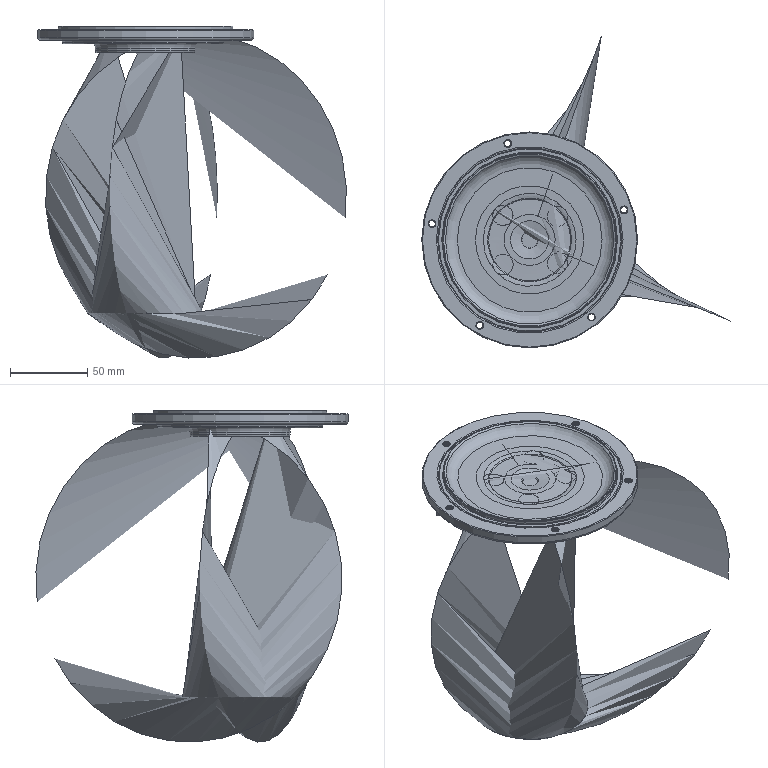NC program | NX | posted with a generic post
Lines 31 to 990 of 33119:
(FIXED_CONTOUR , TOOL : D6R0.5)
N60 T05 M6
N62 G17 G43 G0 G90 X-53.25 Y-3. Z30. S9500 H5 M3
N64 Z3.6
N66 G94 G1 Z2.996 F1000.
N68 Y-2.963 Z2.527
N70 X-53.249 Y-2.853 Z2.069
N72 X-53.246 Y-2.673 Z1.634
N74 X-53.243 Y-2.427 Z1.233
N76 X-53.24 Y-2.121 Z0.875
N78 X-53.235 Y-1.763 Z0.569
N80 X-53.23 Y-1.362 Z0.323
N82 X-53.225 Y-0.927 Z0.143
N84 X-53.219 Y-0.469 Z0.033
N86 X-53.214 Y0. Z-0.004
N88 G2 X29.564 Y44.245 R53.214 F3500.
N90 G1 X30.641 Y43.507
N92 G2 X19.151 Y-49.648 R53.214
N94 G1 X17.927 Y-50.103
N96 G2 X-53.198 Y-1.306 R53.214
N98 G1 X-53.214 Y0.
N100 G2 X-46.923 Y25.081 R53.21
N102 G1 X-46.293 Y26.225
N104 G2 X-28.461 Y44.944 R53.202
N106 G1 X-27.349 Y45.629 Z-0.005
N108 G2 X-2.61 Y53.126 R53.193
N110 G1 X-1.305 Y53.173 Z-0.006
N112 G2 X25.069 Y46.902 R53.185
N114 G1 X26.213 Y46.272
N116 G2 X44.923 Y28.447 R53.177
N118 G1 X45.608 Y27.336 Z-0.007
N120 G2 X53.101 Y2.609 R53.169
N122 G1 X53.149 Y1.305
N124 G2 X47.481 Y-23.9 R53.161
N126 G1 X46.88 Y-25.058 Z-0.008
N128 G2 X28.434 Y-44.903 R53.152
N130 G1 X27.324 Y-45.587
N132 G2 X2.607 Y-53.076 R53.144
N134 G1 X1.304 Y-53.124 Z-0.009
N136 G2 X-23.889 Y-47.459 R53.136
N138 G1 X-25.046 Y-46.858
N140 G2 X-44.171 Y-29.514 R53.128
N142 G1 X-44.882 Y-28.421 Z-0.01
N144 G2 X-52.972 Y-3.907 R53.12
N146 G1 X-53.052 Y-2.606
N148 G2 X-48.009 Y22.707 R53.112
N150 G1 X-47.437 Y23.878 Z-0.011
N152 G2 X-30.575 Y43.414 R53.104
N154 G1 X-29.5 Y44.151
N156 G2 X-5.204 Y52.836 R53.096
N158 G1 X-3.906 Y52.947 Z-0.012
N160 G2 X21.512 Y48.53 R53.087
N162 G1 X22.696 Y47.987
N164 G2 X42.631 Y31.617 R53.079
N166 G1 X43.393 Y30.561 Z-0.013
N168 G2 X52.493 Y7.787 R53.071
N170 G1 X52.668 Y6.496
N172 G2 X51.139 Y-14.152 R53.064
N174 G1 X50.776 Y-15.403 Z-0.014
N176 G2 X42.614 Y-31.605 R53.058
N178 G1 X41.826 Y-32.641
N180 G2 X30.547 Y-43.373 R53.053
N182 G1 X29.473 Y-44.109 Z-0.015
N184 G2 X16.64 Y-50.368 R53.048
N186 G1 X15.398 Y-50.761
N188 G2 X2.603 Y-52.978 R53.043
N190 G1 X1.302 Y-53.025 Z-0.016
N192 G2 X-10.347 Y-52.019 R53.039
N194 G1 X-11.621 Y-51.749
N196 G2 X-22.675 Y-47.942 R53.036
N198 G1 X-23.844 Y-47.371 Z-0.017
N200 G2 X-32.626 Y-41.806 R53.032
N202 G1 X-33.642 Y-40.993
N204 G2 X-40.99 Y-33.64 R53.028
N206 G1 X-41.803 Y-32.624 Z-0.018
N208 G2 X-47.362 Y-23.84 R53.025
N210 G1 X-47.932 Y-22.67
N212 G2 X-51.1 Y-14.141 R53.022
N214 G1 X-51.431 Y-12.883 Z-0.019
N216 G2 X-52.874 Y-3.9 R53.019
N218 G1 X-52.953 Y-2.601 Z-0.02
N220 G2 X-52.615 Y6.489 R53.016
N222 G1 X-52.44 Y7.779
N224 G2 X-50.729 Y15.388 R53.013
N226 G1 X-50.335 Y16.629 Z-0.021
N228 G2 X-47.349 Y23.833 R53.01
N230 G1 X-46.749 Y24.988
N232 G2 X-42.575 Y31.576 R53.007
N234 G1 X-41.787 Y32.611 Z-0.022
N236 G2 X-36.548 Y38.388 R53.004
N238 G1 X-35.595 Y39.273
N240 G2 X-29.446 Y44.068 R53.002
N242 G1 X-28.355 Y44.777 Z-0.023
N244 G2 X-21.477 Y48.451 R52.999
N246 G1 X-20.281 Y48.963
N248 G2 X-12.877 Y51.407 R52.996
N250 G1 X-11.611 Y51.707 Z-0.024
N252 G2 X-3.898 Y52.849 R52.994
N254 G1 X-2.6 Y52.928
N256 G2 X5.194 Y52.735 R52.991
N258 G1 X6.486 Y52.591 Z-0.025
N260 G2 X14.132 Y51.068 R52.988
N262 G1 X15.381 Y50.705
N264 G2 X22.654 Y47.897 R52.986
N266 G1 X23.822 Y47.327 Z-0.026
N268 G2 X30.507 Y43.317 R52.983
N270 G1 X31.561 Y42.555
N272 G2 X37.462 Y37.462 R52.98
N274 G1 X38.37 Y36.531 Z-0.027
N276 G2 X43.313 Y30.504 R52.977
N278 G1 X44.048 Y29.432
N280 G2 X47.888 Y22.649 R52.975
N282 G1 X48.429 Y21.467 Z-0.028
N284 G2 X51.052 Y14.128 R52.972
N286 G1 X51.383 Y12.871
N288 G2 X52.713 Y5.192 R52.969
N290 G1 X52.824 Y3.897 Z-0.029
N292 G2 X52.822 Y-3.896 R52.967
N294 G1 X52.71 Y-5.191
N296 G2 X51.376 Y-12.869 R52.964
N298 G1 X51.044 Y-14.126 Z-0.03
N300 G2 X48.417 Y-21.462 R52.961
N302 G1 X47.875 Y-22.643
N304 G2 X44.032 Y-29.422 R52.959
N306 G1 X43.297 Y-30.493 Z-0.031
N308 G2 X38.352 Y-36.514 R52.956
N310 G1 X37.444 Y-37.444
N312 G2 X31.543 Y-42.531 R52.953
N314 G1 X30.49 Y-43.292 Z-0.032
N316 G2 X23.807 Y-47.296 R52.95
N318 G1 X22.639 Y-47.865
N320 G2 X15.37 Y-50.667 R52.948
N322 G1 X14.121 Y-51.028 Z-0.033
N324 G2 X6.481 Y-52.546 R52.945
N326 G1 X5.189 Y-52.689
N328 G2 X-2.598 Y-52.877 R52.942
N330 G1 X-3.895 Y-52.797 Z-0.034
N332 G2 X-11.599 Y-51.652 R52.94
N334 G1 X-12.863 Y-51.352
N336 G2 X-20.258 Y-48.906 R52.937
N338 G1 X-21.452 Y-48.394 Z-0.035
N340 G2 X-28.319 Y-44.721 R52.934
N342 G1 X-29.408 Y-44.012 Z-0.036
N344 G2 X-35.546 Y-39.219 R52.932
N346 G1 X-36.497 Y-38.334
N348 G2 X-41.725 Y-32.563 R52.929
N350 G1 X-42.512 Y-31.529 Z-0.037
N352 G2 X-46.676 Y-24.949 R52.926
N354 G1 X-47.274 Y-23.796
N356 G2 X-50.251 Y-16.601 R52.923
N358 G1 X-50.643 Y-15.362 Z-0.038
N360 G2 X-52.347 Y-7.765 R52.921
N362 G1 X-52.521 Y-6.478
N364 G2 X-52.901 Y1.299 R52.918
N366 G1 X-52.853 Y2.596 Z-0.039
N368 G2 X-51.897 Y10.323 R52.915
N370 G1 X-51.628 Y11.593
N372 G2 X-49.366 Y19.043 R52.913
N374 G1 X-48.884 Y20.248 Z-0.04
N376 G2 X-45.381 Y27.201 R52.91
N378 G1 X-44.7 Y28.306
N380 G2 X-40.061 Y34.557 R52.907
N382 G1 X-39.201 Y35.529 Z-0.041
N384 G2 X-33.562 Y40.895 R52.905
N386 G1 X-32.548 Y41.706
N388 G2 X-26.075 Y46.028 R52.902
N390 G1 X-24.937 Y46.654 Z-0.042
N392 G2 X-17.821 Y49.806 R52.899
N394 G1 X-16.593 Y50.228
N396 G2 X-9.043 Y52.117 R52.896
N398 G1 X-7.761 Y52.322 Z-0.043
N400 G2 X0. Y52.893 R52.894
N402 G1 X1.298 Y52.876
N404 G2 X9.042 Y52.111 R52.891
N406 G1 X10.318 Y51.873 Z-0.044
N408 G2 X17.817 Y49.796 R52.888
N410 G1 X19.034 Y49.343
N412 G2 X26.067 Y46.014 R52.886
N414 G1 X27.188 Y45.36 Z-0.045
N416 G2 X33.548 Y40.878 R52.883
N418 G1 X34.541 Y40.042
N420 G2 X40.041 Y34.539 R52.88
N422 G1 X40.876 Y33.546 Z-0.046
N424 G2 X45.354 Y27.184 R52.878
N426 G1 X46.007 Y26.062
N428 G2 X49.331 Y19.029 R52.875
N430 G1 X49.783 Y17.812 Z-0.047
N432 G2 X51.855 Y10.315 R52.872
N434 G1 X52.092 Y9.039
N436 G2 X52.852 Y1.297 R52.869
N438 G1 X52.868 Y0. Z-0.048
N440 G2 X52.293 Y-7.757 R52.867
N442 G1 X52.087 Y-9.038
N444 G2 X50.195 Y-16.582 R52.864
N446 G1 X49.772 Y-17.809 Z-0.049
N448 G2 X46.619 Y-24.918 R52.861
N450 G1 X45.993 Y-26.055
N452 G2 X41.67 Y-32.52 R52.859
N454 G1 X40.859 Y-33.532 Z-0.05
N456 G2 X35.495 Y-39.163 R52.856
N458 G1 X34.523 Y-40.022
N460 G2 X28.276 Y-44.652 R52.853
N462 G1 X27.171 Y-45.332 Z-0.051
N464 G2 X20.225 Y-48.826 R52.851
N466 G1 X19.02 Y-49.308 Z-0.052
N468 G2 X11.579 Y-51.563 R52.848
N470 G1 X10.31 Y-51.831
N472 G2 X2.593 Y-52.78 R52.845
N474 G1 X1.297 Y-52.828 Z-0.053
N476 G2 X-6.468 Y-52.444 R52.842
N478 G1 X-7.753 Y-52.269
N480 G2 X-15.338 Y-50.563 R52.84
N482 G1 X-16.574 Y-50.171 Z-0.054
N484 G2 X-23.756 Y-47.194 R52.837
N486 G1 X-24.906 Y-46.597
N488 G2 X-31.473 Y-42.436 R52.834
N490 G1 X-32.504 Y-41.651 Z-0.055
N492 G2 X-38.262 Y-36.429 R52.832
N494 G1 X-39.145 Y-35.479
N496 G2 X-43.925 Y-29.35 R52.829
N498 G1 X-44.631 Y-28.263 Z-0.056
N500 G2 X-48.293 Y-21.407 R52.826
N502 G1 X-48.804 Y-20.215
N504 G2 X-51.239 Y-12.835 R52.824
N506 G1 X-51.539 Y-11.573 Z-0.057
N508 G2 X-52.677 Y-3.886 R52.821
N510 G1 X-52.756 Y-2.592
N512 G2 X-52.563 Y5.177 R52.818
N514 G1 X-52.419 Y6.465 Z-0.058
N516 G2 X-50.901 Y14.086 R52.815
N518 G1 X-50.54 Y15.331
N520 G2 X-48.281 Y21.402 R52.813
N522 G1 X-47.741 Y22.58 Z-0.059
N524 G2 X-44.616 Y28.253 R52.811
N526 G1 X-43.909 Y29.339
N528 G2 X-39.986 Y34.492 R52.808
N530 G1 X-39.127 Y35.463 Z-0.06
N532 G2 X-34.491 Y39.984 R52.806
N534 G1 X-33.499 Y40.819
N536 G2 X-28.249 Y44.611 R52.804
N538 G1 X-27.146 Y45.29 Z-0.061
N540 G2 X-21.397 Y48.271 R52.801
N542 G1 X-20.206 Y48.781 Z-0.062
N544 G2 X-14.082 Y50.886 R52.799
N546 G1 X-12.829 Y51.215
N548 G2 X-6.463 Y52.399 R52.797
N550 G1 X-5.175 Y52.541 Z-0.063
N552 G2 X1.296 Y52.778 R52.795
N554 G1 X2.59 Y52.729
N556 X3.884 Y52.65
N558 X5.175 Y52.538
N560 X6.462 Y52.395 Z-0.064
N562 X7.746 Y52.22
N564 X9.025 Y52.014
N566 X10.299 Y51.776
N568 X11.566 Y51.508
N570 X12.827 Y51.208
N572 X14.08 Y50.877
N574 X15.324 Y50.516
N576 X16.559 Y50.124
N578 X17.784 Y49.703
N580 X18.998 Y49.251 Z-0.065
N582 X20.201 Y48.769
N584 X21.392 Y48.259
N586 X22.569 Y47.719
N588 X23.733 Y47.15
N590 X24.883 Y46.553
N592 X26.018 Y45.928
N594 X27.137 Y45.276
N596 X28.24 Y44.596
N598 X29.326 Y43.889 Z-0.066
N600 X30.394 Y43.156
N602 X31.443 Y42.396
N604 X32.474 Y41.612
N606 X33.485 Y40.802
N608 X34.476 Y39.968
N610 X35.446 Y39.109
N612 X36.395 Y38.227
N614 X37.322 Y37.322
N616 X38.227 Y36.395 Z-0.067
N618 X39.108 Y35.445
N620 X39.966 Y34.475
N622 X40.799 Y33.483
N624 X41.609 Y32.472
N626 X42.393 Y31.441
N628 X43.151 Y30.39
N630 X43.884 Y29.322
N632 X44.59 Y28.236
N634 X45.269 Y27.133 Z-0.068
N636 X45.921 Y26.014
N638 X46.545 Y24.879
N640 X47.141 Y23.729
N642 X47.709 Y22.565
N644 X48.248 Y21.387
N646 X48.758 Y20.196
N648 X49.239 Y18.993
N650 X49.69 Y17.779
N652 X50.111 Y16.554 Z-0.069
N654 X50.501 Y15.319
N656 X50.862 Y14.075
N658 X51.191 Y12.823
N660 X51.49 Y11.563
N662 X51.758 Y10.295
N664 X51.995 Y9.022
N666 X52.2 Y7.743
N668 X52.374 Y6.46 Z-0.07
N670 X52.517 Y5.172
N672 X52.627 Y3.882
N674 X52.706 Y2.589
N676 X52.754 Y1.295
N678 X52.769 Y0.
N680 X52.753 Y-1.295
N682 X52.705 Y-2.589
N684 X52.625 Y-3.882
N686 X52.514 Y-5.172 Z-0.071
N688 X52.37 Y-6.459
N690 X52.196 Y-7.743
N692 X51.99 Y-9.021
N694 X51.752 Y-10.294
N696 X51.484 Y-11.561
N698 X51.184 Y-12.821
N700 X50.854 Y-14.073
N702 X50.493 Y-15.317 Z-0.072
N704 X50.101 Y-16.551
N706 X49.679 Y-17.776
N708 X49.228 Y-18.989
N710 X48.747 Y-20.192
N712 X48.236 Y-21.382
N714 X47.696 Y-22.559
N716 X47.128 Y-23.722
N718 X46.531 Y-24.872 Z-0.073
N720 X45.907 Y-26.006
N722 X45.254 Y-27.124
N724 X44.575 Y-28.227
N726 X43.868 Y-29.312
N728 X43.135 Y-30.379
N730 X42.377 Y-31.429
N732 X41.592 Y-32.459
N734 X40.783 Y-33.47 Z-0.074
N736 X39.949 Y-34.46
N738 X39.091 Y-35.43
N740 X38.209 Y-36.378
N742 X37.305 Y-37.305
N744 X36.378 Y-38.209
N746 X35.429 Y-39.09
N748 X34.459 Y-39.947
N750 X33.468 Y-40.78 Z-0.075
N752 X32.456 Y-41.589
N754 X31.426 Y-42.373
N756 X30.376 Y-43.131
N758 X29.308 Y-43.863
N760 X28.223 Y-44.569
N762 X27.12 Y-45.248
N764 X26.002 Y-45.899
N766 X24.867 Y-46.523 Z-0.076
N768 X23.718 Y-47.119
N770 X22.554 Y-47.687
N772 X21.377 Y-48.226
N774 X20.187 Y-48.735
N776 X18.985 Y-49.216
N778 X17.771 Y-49.666
N780 X16.547 Y-50.087
N782 X15.312 Y-50.478 Z-0.077
N784 X14.069 Y-50.838
N786 X12.817 Y-51.168
N788 X11.557 Y-51.466
N790 X10.291 Y-51.734
N792 X9.018 Y-51.971
N794 X7.74 Y-52.176
N796 X6.457 Y-52.35
N798 X5.17 Y-52.492 Z-0.078
N800 X3.88 Y-52.603
N802 X2.588 Y-52.682
N804 X1.294 Y-52.729
N806 X0. Y-52.744
N808 X-1.294 Y-52.728
N810 X-2.588 Y-52.68
N812 X-3.88 Y-52.6
N814 X-5.17 Y-52.489 Z-0.079
N816 X-6.456 Y-52.346
N818 X-7.739 Y-52.171
N820 X-9.017 Y-51.965
N822 X-10.289 Y-51.728
N824 X-11.556 Y-51.46
N826 X-12.815 Y-51.16
N828 X-14.067 Y-50.83 Z-0.08
N830 X-15.31 Y-50.469
N832 X-16.543 Y-50.078
N834 X-17.767 Y-49.656
N836 X-18.98 Y-49.205
N838 X-20.182 Y-48.724
N840 X-21.372 Y-48.214
N842 X-22.548 Y-47.674
N844 X-23.711 Y-47.106 Z-0.081
N846 X-24.86 Y-46.51
N848 X-25.994 Y-45.885
N850 X-27.112 Y-45.233
N852 X-28.213 Y-44.554
N854 X-29.298 Y-43.848
N856 X-30.365 Y-43.115
N858 X-31.414 Y-42.357
N860 X-32.444 Y-41.573 Z-0.082
N862 X-33.454 Y-40.764
N864 X-34.444 Y-39.93
N866 X-35.413 Y-39.073
N868 X-36.361 Y-38.191
N870 X-37.287 Y-37.287
N872 X-38.191 Y-36.361
N874 X-39.071 Y-35.412
N876 X-39.928 Y-34.442 Z-0.083
N878 X-40.761 Y-33.452
N880 X-41.57 Y-32.441
N882 X-42.353 Y-31.411
N884 X-43.111 Y-30.362
N886 X-43.843 Y-29.295
N888 X-44.548 Y-28.21
N890 X-45.227 Y-27.108
N892 X-45.878 Y-25.989 Z-0.084
N894 X-46.502 Y-24.856
N896 X-47.097 Y-23.707
N898 X-47.664 Y-22.544
N900 X-48.203 Y-21.367
N902 X-48.712 Y-20.177
N904 X-49.193 Y-18.976
N906 X-49.643 Y-17.763
N908 X-50.064 Y-16.539 Z-0.085
N910 X-50.454 Y-15.305
N912 X-50.814 Y-14.062
N914 X-51.144 Y-12.811
N916 X-51.442 Y-11.552
N918 X-51.71 Y-10.286
N920 X-51.946 Y-9.014
N922 X-52.151 Y-7.736
N924 X-52.325 Y-6.454 Z-0.086
N926 X-52.467 Y-5.168
N928 X-52.578 Y-3.878
N930 X-52.657 Y-2.587
N932 X-52.704 Y-1.294
N934 X-52.72 Y0.
N936 X-52.704 Y1.294
N938 X-52.656 Y2.587
N940 X-52.576 Y3.878 Z-0.087
N942 X-52.464 Y5.167
N944 X-52.321 Y6.453
N946 X-52.147 Y7.735
N948 X-51.941 Y9.013
N950 X-51.704 Y10.285
N952 X-51.435 Y11.55
N954 X-51.136 Y12.809
N956 X-50.806 Y14.06 Z-0.088
N958 X-50.445 Y15.302
N960 X-50.054 Y16.536
N962 X-49.633 Y17.759
N964 X-49.182 Y18.971
N966 X-48.701 Y20.173
N968 X-48.191 Y21.362
N970 X-47.652 Y22.538
N972 X-47.084 Y23.7 Z-0.089
N974 X-46.488 Y24.848
N976 X-45.864 Y25.981
N978 X-45.212 Y27.099
N980 X-44.533 Y28.2
N982 X-43.827 Y29.284
N984 X-43.095 Y30.351
N986 X-42.337 Y31.399
N988 X-41.553 Y32.428 Z-0.09
N990 X-40.745 Y33.438
N992 X-39.911 Y34.428
N994 X-39.054 Y35.397
N996 X-38.174 Y36.344
N998 X-37.27 Y37.27
N1000 X-36.344 Y38.173
N1002 X-35.396 Y39.053
N1004 X-34.426 Y39.91 Z-0.091
N1006 X-33.436 Y40.742
N1008 X-32.426 Y41.55
N1010 X-31.396 Y42.333
N1012 X-30.348 Y43.091
N1014 X-29.281 Y43.822
N1016 X-28.196 Y44.527
N1018 X-27.095 Y45.205
N1020 X-25.977 Y45.856 Z-0.092
N1022 X-24.844 Y46.48
N1024 X-23.696 Y47.075
N1026 X-22.533 Y47.642
N1028 X-21.357 Y48.18
N1030 X-20.168 Y48.69
N1032 X-18.967 Y49.17
N1034 X-17.754 Y49.62
N1036 X-16.531 Y50.04 Z-0.093
N1038 X-15.298 Y50.431
N1040 X-14.056 Y50.79
N1042 X-12.805 Y51.12
N1044 X-11.546 Y51.418
N1046 X-10.281 Y51.686
N1048 X-9.009 Y51.922
N1050 X-7.732 Y52.127
N1052 X-6.451 Y52.301 Z-0.094
N1054 X-5.165 Y52.443
N1056 X-3.877 Y52.553
N1058 X-2.586 Y52.632
N1060 X-1.293 Y52.68
N1062 X0. Y52.695
N1064 X1.293 Y52.679
N1066 X2.586 Y52.631
N1068 X3.876 Y52.551 Z-0.095
N1070 X5.165 Y52.44
N1072 X6.45 Y52.297
N1074 X7.732 Y52.122
N1076 X9.008 Y51.917
N1078 X10.28 Y51.68
N1080 X11.545 Y51.411
N1082 X12.803 Y51.112
N1084 X14.053 Y50.782 Z-0.096
N1086 X15.295 Y50.422
N1088 X16.528 Y50.031
N1090 X17.751 Y49.61
N1092 X18.963 Y49.159
N1094 X20.163 Y48.678
N1096 X21.352 Y48.168
N1098 X22.527 Y47.63
N1100 X23.689 Y47.062 Z-0.097
N1102 X24.837 Y46.466
N1104 X25.969 Y45.842
N1106 X27.086 Y45.191
N1108 X28.187 Y44.512
N1110 X29.271 Y43.807
N1112 X30.337 Y43.075
N1114 X31.384 Y42.317
N1116 X32.413 Y41.534 Z-0.098
N1118 X33.423 Y40.726
N1120 X34.412 Y39.893
N1122 X35.38 Y39.036
N1124 X36.327 Y38.156
N1126 X37.252 Y37.252
N1128 X38.155 Y36.327
N1130 X39.035 Y35.379
N1132 X39.891 Y34.41 Z-0.099
N1134 X40.723 Y33.421
N1136 X41.531 Y32.411
N1138 X42.313 Y31.382
N1140 X43.07 Y30.334
N1142 X43.802 Y29.267
N1144 X44.506 Y28.183
N1146 X45.184 Y27.082
N1148 X45.835 Y25.965 Z-0.1
N1150 X46.458 Y24.832
N1152 X47.053 Y23.685
N1154 X47.62 Y22.522
N1156 X48.158 Y21.347
N1158 X48.667 Y20.158
N1160 X49.147 Y18.958
N1162 X49.597 Y17.746
N1164 X50.017 Y16.523 Z-0.101
N1166 X50.407 Y15.291
N1168 X50.767 Y14.049
N1170 X51.096 Y12.799
N1172 X51.394 Y11.541
N1174 X51.661 Y10.276
N1176 X51.898 Y9.005
N1178 X52.103 Y7.729
N1180 X52.276 Y6.448 Z-0.102
N1182 X52.418 Y5.163
N1184 X52.529 Y3.875
N1186 X52.608 Y2.584
N1188 X52.655 Y1.293
N1190 X52.67 Y0.
N1192 X52.654 Y-1.293
N1194 X52.606 Y-2.584
N1196 X52.527 Y-3.875 Z-0.103
N1198 X52.415 Y-5.162
N1200 X52.272 Y-6.447
N1202 X52.098 Y-7.728
N1204 X51.892 Y-9.004
N1206 X51.655 Y-10.275
N1208 X51.387 Y-11.539
N1210 X51.088 Y-12.797
N1212 X50.758 Y-14.047 Z-0.104
N1214 X50.398 Y-15.288
N1216 X50.007 Y-16.52
N1218 X49.586 Y-17.742
N1220 X49.136 Y-18.954
N1222 X48.655 Y-20.154
N1224 X48.146 Y-21.342
N1226 X47.607 Y-22.517
N1228 X47.04 Y-23.678 Z-0.105
N1230 X46.444 Y-24.825
N1232 X45.821 Y-25.957
N1234 X45.17 Y-27.074
N1236 X44.491 Y-28.174
N1238 X43.786 Y-29.257
N1240 X43.055 Y-30.323
N1242 X42.297 Y-31.37
N1244 X41.514 Y-32.398 Z-0.106
N1246 X40.706 Y-33.407
N1248 X39.874 Y-34.396
N1250 X39.018 Y-35.364
N1252 X38.138 Y-36.31
N1254 X37.235 Y-37.235
N1256 X36.31 Y-38.137
N1258 X35.362 Y-39.017
N1260 X34.394 Y-39.872 Z-0.107
N1262 X33.405 Y-40.704
N1264 X32.396 Y-41.511
N1266 X31.367 Y-42.294
N1268 X30.319 Y-43.05
N1270 X29.254 Y-43.781
N1272 X28.17 Y-44.485
N1274 X27.07 Y-45.163
N1276 X25.953 Y-45.813 Z-0.108
N1278 X24.821 Y-46.436
N1280 X23.673 Y-47.031
N1282 X22.512 Y-47.597
N1284 X21.337 Y-48.135
N1286 X20.149 Y-48.644
N1288 X18.949 Y-49.123
N1290 X17.738 Y-49.573
N1292 X16.516 Y-49.993 Z-0.109
N1294 X15.284 Y-50.383
N1296 X14.042 Y-50.743
N1298 X12.793 Y-51.072
N1300 X11.536 Y-51.37
N1302 X10.271 Y-51.637
N1304 X9.001 Y-51.873
N1306 X7.725 Y-52.078
N1308 X6.445 Y-52.252 Z-0.11
N1310 X5.16 Y-52.394
N1312 X3.873 Y-52.504
N1314 X2.583 Y-52.583
N1316 X1.292 Y-52.63
N1318 X0. Y-52.646
N1320 X-1.292 Y-52.629
N1322 X-2.583 Y-52.582
N1324 X-3.873 Y-52.502 Z-0.111
N1326 X-5.16 Y-52.391
N1328 X-6.444 Y-52.248
N1330 X-7.724 Y-52.074
N1332 X-9. Y-51.868
N1334 X-10.27 Y-51.631
N1336 X-11.534 Y-51.363
N1338 X-12.791 Y-51.064
N1340 X-14.04 Y-50.735 Z-0.112
N1342 X-15.281 Y-50.374
N1344 X-16.512 Y-49.984
N1346 X-17.734 Y-49.563
N1348 X-18.945 Y-49.113
N1350 X-20.144 Y-48.633
N1352 X-21.332 Y-48.123
N1354 X-22.506 Y-47.585 Z-0.113
N1356 X-23.667 Y-47.018
N1358 X-24.813 Y-46.423
N1360 X-25.945 Y-45.799
N1362 X-27.061 Y-45.148
N1364 X-28.161 Y-44.47
N1366 X-29.243 Y-43.766
N1368 X-30.308 Y-43.034
N1370 X-31.355 Y-42.277 Z-0.114
N1372 X-32.383 Y-41.495
N1374 X-33.391 Y-40.687
N1376 X-34.379 Y-39.855
N1378 X-35.347 Y-38.999
N1380 X-36.293 Y-38.12
N1382 X-37.217 Y-37.217
N1384 X-38.119 Y-36.293
N1386 X-38.998 Y-35.346 Z-0.115
N1388 X-39.854 Y-34.378
N1390 X-40.685 Y-33.389
N1392 X-41.492 Y-32.38
N1394 X-42.274 Y-31.352
N1396 X-43.03 Y-30.305
N1398 X-43.761 Y-29.24
N1400 X-44.465 Y-28.157
N1402 X-45.142 Y-27.057 Z-0.116
N1404 X-45.792 Y-25.941
N1406 X-46.414 Y-24.809
N1408 X-47.009 Y-23.662
N1410 X-47.575 Y-22.501
N1412 X-48.113 Y-21.327
N1414 X-48.621 Y-20.14
N1416 X-49.1 Y-18.94
N1418 X-49.55 Y-17.729 Z-0.117
N1420 X-49.97 Y-16.508
N1422 X-50.36 Y-15.276
N1424 X-50.719 Y-14.036
N1426 X-51.048 Y-12.787
N1428 X-51.346 Y-11.53
N1430 X-51.613 Y-10.267
N1432 X-51.849 Y-8.997
N1434 X-52.054 Y-7.722 Z-0.118
N1436 X-52.227 Y-6.442
N1438 X-52.369 Y-5.158
N1440 X-52.48 Y-3.871
N1442 X-52.558 Y-2.582
N1444 X-52.606 Y-1.291
N1446 X-52.621 Y0.
N1448 X-52.605 Y1.291
N1450 X-52.557 Y2.582 Z-0.119
N1452 X-52.477 Y3.871
N1454 X-52.366 Y5.158
N1456 X-52.223 Y6.441
N1458 X-52.049 Y7.721
N1460 X-51.844 Y8.996
N1462 X-51.607 Y10.265
N1464 X-51.339 Y11.529
N1466 X-51.04 Y12.785 Z-0.12
N1468 X-50.711 Y14.034
N1470 X-50.351 Y15.274
N1472 X-49.96 Y16.505
N1474 X-49.54 Y17.726
N1476 X-49.09 Y18.936
N1478 X-48.61 Y20.135
N1480 X-48.101 Y21.322
N1482 X-47.563 Y22.495 Z-0.121
N1484 X-46.996 Y23.656
N1486 X-46.401 Y24.802
N1488 X-45.778 Y25.933
N1490 X-45.127 Y27.048
N1492 X-44.45 Y28.147
N1494 X-43.745 Y29.229
N1496 X-43.014 Y30.294
N1498 X-42.258 Y31.34 Z-0.122
N1500 X-41.475 Y32.368
N1502 X-40.668 Y33.376
N1504 X-39.837 Y34.363
N1506 X-38.981 Y35.33
N1508 X-38.102 Y36.276
N1510 X-37.2 Y37.2
N1512 X-36.276 Y38.101
N1514 X-35.329 Y38.98 Z-0.123
N1516 X-34.362 Y39.835
N1518 X-33.374 Y40.666
N1520 X-32.365 Y41.472
N1522 X-31.338 Y42.254
N1524 X-30.291 Y43.01
N1526 X-29.226 Y43.74
N1528 X-28.144 Y44.444
N1530 X-27.044 Y45.121 Z-0.124
N1532 X-25.929 Y45.77
N1534 X-24.797 Y46.393
N1536 X-23.651 Y46.987
N1538 X-22.491 Y47.553
N1540 X-21.317 Y48.09
N1542 X-20.13 Y48.598
N1544 X-18.931 Y49.077
N1546 X-17.721 Y49.527 Z-0.125
N1548 X-16.5 Y49.946
N1550 X-15.269 Y50.336
N1552 X-14.029 Y50.695
N1554 X-12.781 Y51.024
N1556 X-11.525 Y51.322
N1558 X-10.262 Y51.589
N1560 X-8.992 Y51.825
N1562 X-7.718 Y52.029 Z-0.126
N1564 X-6.439 Y52.203
N1566 X-5.156 Y52.345
N1568 X-3.869 Y52.455
N1570 X-2.581 Y52.534
N1572 X-1.291 Y52.581
N1574 X0. Y52.596
N1576 X1.291 Y52.58
N1578 X2.581 Y52.532 Z-0.127
N1580 X3.869 Y52.453
N1582 X5.155 Y52.342
N1584 X6.438 Y52.199
N1586 X7.717 Y52.025
N1588 X8.992 Y51.819
N1590 X10.261 Y51.583
N1592 X11.523 Y51.315
N1594 X12.779 Y51.016 Z-0.128
N1596 X14.027 Y50.687
N1598 X15.267 Y50.327
N1600 X16.497 Y49.937
N1602 X17.717 Y49.517
N1604 X18.927 Y49.067
N1606 X20.125 Y48.587
N1608 X21.312 Y48.078
N1610 X22.485 Y47.54 Z-0.129
N1612 X23.645 Y46.974
N1614 X24.79 Y46.379
N1616 X25.921 Y45.756
N1618 X27.036 Y45.106
N1620 X28.134 Y44.429
N1622 X29.216 Y43.725
N1624 X30.28 Y42.994
N1626 X31.326 Y42.238 Z-0.13
N1628 X32.353 Y41.456
N1630 X33.36 Y40.649
N1632 X34.347 Y39.818
N1634 X35.314 Y38.963
N1636 X36.259 Y38.084
N1638 X37.183 Y37.182
N1640 X38.084 Y36.259
N1642 X38.962 Y35.313 Z-0.131
N1644 X39.816 Y34.346
N1646 X40.647 Y33.358
N1648 X41.453 Y32.35
N1650 X42.234 Y31.323
N1652 X42.99 Y30.277
N1654 X43.719 Y29.212
N1656 X44.423 Y28.13
N1658 X45.1 Y27.032 Z-0.132
N1660 X45.749 Y25.916
N1662 X46.371 Y24.786
N1664 X46.965 Y23.64
N1666 X47.531 Y22.48
N1668 X48.068 Y21.307
N1670 X48.576 Y20.121
N1672 X49.054 Y18.922 Z-0.133
N1674 X49.504 Y17.713
N1676 X49.923 Y16.492
N1678 X50.312 Y15.262
N1680 X50.671 Y14.023
N1682 X51. Y12.775
N1684 X51.298 Y11.519
N1686 X51.565 Y10.257
N1688 X51.8 Y8.988 Z-0.134
N1690 X52.005 Y7.714
N1692 X52.178 Y6.436
N1694 X52.32 Y5.153
N1696 X52.43 Y3.867
N1698 X52.509 Y2.58
N1700 X52.556 Y1.29
N1702 X52.572 Y0. Z-0.135
N1704 X52.555 Y-1.29
N1706 X52.508 Y-2.58
N1708 X52.428 Y-3.867
N1710 X52.317 Y-5.153
N1712 X52.174 Y-6.435
N1714 X52. Y-7.714
N1716 X51.795 Y-8.987 Z-0.136
N1718 X51.559 Y-10.256
N1720 X51.291 Y-11.518
N1722 X50.992 Y-12.773
N1724 X50.663 Y-14.02
N1726 X50.304 Y-15.259
N1728 X49.914 Y-16.489
N1730 X49.493 Y-17.709
N1732 X49.044 Y-18.918 Z-0.137
N1734 X48.564 Y-20.116
N1736 X48.056 Y-21.302
N1738 X47.518 Y-22.474
N1740 X46.952 Y-23.634
N1742 X46.357 Y-24.778
N1744 X45.735 Y-25.908
N1746 X45.085 Y-27.023 Z-0.138
N1748 X44.408 Y-28.121
N1750 X43.704 Y-29.202
N1752 X42.974 Y-30.266
N1754 X42.218 Y-31.311
N1756 X41.436 Y-32.337
N1758 X40.63 Y-33.344 Z-0.139
N1760 X39.799 Y-34.331
N1762 X38.944 Y-35.297
N1764 X38.066 Y-36.242
N1766 X37.165 Y-37.165
N1768 X36.242 Y-38.066
N1770 X35.296 Y-38.943
N1772 X34.33 Y-39.798 Z-0.14
N1774 X33.342 Y-40.628
N1776 X32.335 Y-41.433
N1778 X31.308 Y-42.214
N1780 X30.263 Y-42.97
N1782 X29.199 Y-43.699
N1784 X28.117 Y-44.402
N1786 X27.019 Y-45.078 Z-0.141
N1788 X25.904 Y-45.727
N1790 X24.774 Y-46.349
N1792 X23.629 Y-46.943
N1794 X22.47 Y-47.508
N1796 X21.297 Y-48.045
N1798 X20.111 Y-48.553 Z-0.142
N1800 X18.914 Y-49.031
N1802 X17.704 Y-49.48
N1804 X16.485 Y-49.9
N1806 X15.255 Y-50.289
N1808 X14.016 Y-50.648
N1810 X12.769 Y-50.976
N1812 X11.514 Y-51.274 Z-0.143
N1814 X10.252 Y-51.54
N1816 X8.984 Y-51.776
N1818 X7.711 Y-51.981
N1820 X6.433 Y-52.154
N1822 X5.151 Y-52.295
N1824 X3.866 Y-52.406 Z-0.144
N1826 X2.578 Y-52.484
N1828 X1.29 Y-52.532
N1830 X0. Y-52.547
N1832 X-1.29 Y-52.531
N1834 X-2.578 Y-52.483
N1836 X-3.866 Y-52.403 Z-0.145
N1838 X-5.15 Y-52.292
N1840 X-6.432 Y-52.15
N1842 X-7.71 Y-51.976
N1844 X-8.983 Y-51.771
N1846 X-10.251 Y-51.534
N1848 X-11.512 Y-51.267 Z-0.146
N1850 X-12.767 Y-50.968
N1852 X-14.014 Y-50.639
N1854 X-15.252 Y-50.28
N1856 X-16.481 Y-49.89
N1858 X-17.701 Y-49.47
N1860 X-18.909 Y-49.021 Z-0.147
N1862 X-20.107 Y-48.541
N1864 X-21.292 Y-48.033
N1866 X-22.464 Y-47.496
N1868 X-23.622 Y-46.93
N1870 X-24.767 Y-46.336
N1872 X-25.896 Y-45.713 Z-0.148
N1874 X-27.01 Y-45.064
N1876 X-28.108 Y-44.387
N1878 X-29.188 Y-43.684
N1880 X-30.251 Y-42.954
N1882 X-31.296 Y-42.198
N1884 X-32.322 Y-41.417 Z-0.149
N1886 X-33.329 Y-40.611
N1888 X-34.315 Y-39.781
N1890 X-35.281 Y-38.926
N1892 X-36.225 Y-38.048
N1894 X-37.148 Y-37.148
N1896 X-38.048 Y-36.224 Z-0.15
N1898 X-38.925 Y-35.28
N1900 X-39.779 Y-34.313
N1902 X-40.609 Y-33.327
N1904 X-41.414 Y-32.32
N1906 X-42.194 Y-31.293
N1908 X-42.949 Y-30.248 Z-0.151
N1910 X-43.678 Y-29.185
N1912 X-44.381 Y-28.104
N1914 X-45.057 Y-27.006
N1916 X-45.706 Y-25.892
N1918 X-46.327 Y-24.762 Z-0.152
N1920 X-46.921 Y-23.618
N1922 X-47.486 Y-22.459
N1924 X-48.022 Y-21.287
N1926 X-48.53 Y-20.102
N1928 X-49.008 Y-18.905
N1930 X-49.457 Y-17.696 Z-0.153
N1932 X-49.876 Y-16.477
N1934 X-50.265 Y-15.248
N1936 X-50.624 Y-14.01
N1938 X-50.952 Y-12.763
N1940 X-51.249 Y-11.509
N1942 X-51.516 Y-10.247 Z-0.154
N1944 X-51.752 Y-8.98
N1946 X-51.956 Y-7.707
N1948 X-52.129 Y-6.43
N1950 X-52.271 Y-5.148
N1952 X-52.381 Y-3.864 Z-0.155
N1954 X-52.46 Y-2.577
N1956 X-52.507 Y-1.289
N1958 X-52.522 Y0.
N1960 X-52.506 Y1.289
N1962 X-52.458 Y2.577
N1964 X-52.379 Y3.864 Z-0.156
N1966 X-52.268 Y5.148
N1968 X-52.125 Y6.429
N1970 X-51.952 Y7.706
N1972 X-51.746 Y8.979